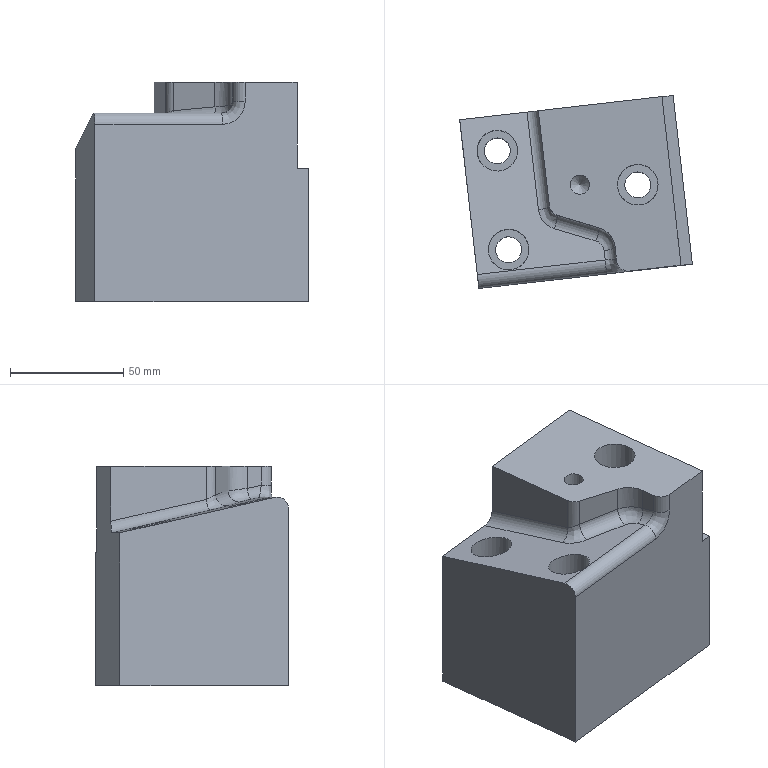Part | NX | features solid 2 | 1 solid | 37 faces | box 102.88 x 85.272 x 97 mm | volume 557494 mm3 | cylinder 16 | plane 15 | spline 3 | cone 3 | commonest cylinder face diameters 10 x6 8.5 x3 11.5 x3 18 x3 20 x1
STEP:
#1=CARTESIAN_POINT('',(2285.765,326.679,-55.281));
#2=VERTEX_POINT('',#1);
#3=CARTESIAN_POINT('',(2285.765,326.679,-31.));
#4=VERTEX_POINT('',#3);
#5=CARTESIAN_POINT('',(2285.765,326.679,-37.));
#6=DIRECTION('',(0.,0.,1.));
#7=VECTOR('',#6,1000.);
#8=LINE('',#5,#7);
#9=EDGE_CURVE('',#2,#4,#8,.T.);
#10=ORIENTED_EDGE('',*,*,#9,.T.);
#11=CARTESIAN_POINT('',(2340.433,332.908,-31.));
#12=VERTEX_POINT('',#11);
#13=CARTESIAN_POINT('',(2360.305,335.172,-31.));
#14=DIRECTION('',(0.9936,0.1132,0.));
#15=VECTOR('',#14,1000.);
#16=LINE('',#13,#15);
#17=EDGE_CURVE('',#4,#12,#16,.T.);
#18=ORIENTED_EDGE('',*,*,#17,.T.);
#19=CARTESIAN_POINT('',(2340.433,332.908,-69.));
#20=VERTEX_POINT('',#19);
#21=CARTESIAN_POINT('',(2340.433,332.908,-37.));
#22=DIRECTION('',(0.,0.,1.));
#23=VECTOR('',#22,1000.);
#24=LINE('',#21,#23);
#25=EDGE_CURVE('',#20,#12,#24,.T.);
#26=ORIENTED_EDGE('',*,*,#25,.F.);
#27=CARTESIAN_POINT('',(2345.401,333.474,-69.));
#28=VERTEX_POINT('',#27);
#29=CARTESIAN_POINT('',(2360.305,335.172,-69.));
#30=DIRECTION('',(0.9936,0.1132,0.));
#31=VECTOR('',#30,1000.);
#32=LINE('',#29,#31);
#33=EDGE_CURVE('',#20,#28,#32,.T.);
#34=ORIENTED_EDGE('',*,*,#33,.T.);
#35=CARTESIAN_POINT('',(2345.401,333.474,-128.));
#36=VERTEX_POINT('',#35);
#37=CARTESIAN_POINT('',(2345.401,333.474,-37.));
#38=DIRECTION('',(0.,0.,1.));
#39=VECTOR('',#38,1000.);
#40=LINE('',#37,#39);
#41=EDGE_CURVE('',#36,#28,#40,.T.);
#42=ORIENTED_EDGE('',*,*,#41,.F.);
#43=CARTESIAN_POINT('',(2251.012,322.719,-128.));
#44=VERTEX_POINT('',#43);
#45=CARTESIAN_POINT('',(2360.305,335.172,-128.));
#46=DIRECTION('',(0.9936,0.1132,0.));
#47=VECTOR('',#46,1000.);
#48=LINE('',#45,#47);
#49=EDGE_CURVE('',#44,#36,#48,.T.);
#50=ORIENTED_EDGE('',*,*,#49,.F.);
#51=CARTESIAN_POINT('',(2251.012,322.719,-60.413));
#52=VERTEX_POINT('',#51);
#53=CARTESIAN_POINT('',(2251.012,322.719,-45.));
#54=DIRECTION('',(0.,0.,-1.));
#55=VECTOR('',#54,1000.);
#56=LINE('',#53,#55);
#57=EDGE_CURVE('',#52,#44,#56,.T.);
#58=ORIENTED_EDGE('',*,*,#57,.F.);
#59=CARTESIAN_POINT('',(2280.794,326.113,-60.413));
#60=VERTEX_POINT('',#59);
#61=CARTESIAN_POINT('',(2360.305,335.172,-60.413));
#62=DIRECTION('',(0.9936,0.1132,-0.000000001));
#63=VECTOR('',#62,1000.);
#64=LINE('',#61,#63);
#65=EDGE_CURVE('',#52,#60,#64,.T.);
#66=ORIENTED_EDGE('',*,*,#65,.T.);
#67=CARTESIAN_POINT('',(2280.797,326.113,-55.285));
#68=DIRECTION('',(-0.1132,0.9936,0.));
#69=DIRECTION('',(-0.01222,-0.001392,-0.9999));
#70=AXIS2_PLACEMENT_3D('',#67,#68,#69);
#71=ELLIPSE('',#70,5.128,5.);
#72=EDGE_CURVE('',#2,#60,#71,.T.);
#73=ORIENTED_EDGE('',*,*,#72,.F.);
#74=EDGE_LOOP('',(#10,#18,#26,#34,#42,#50,#58,#66,#73));
#75=FACE_BOUND('',#74,.T.);
#76=CARTESIAN_POINT('',(2360.305,335.172,-37.));
#77=DIRECTION('',(-0.1132,0.9936,0.));
#78=DIRECTION('',(-0.9936,-0.1132,0.));
#79=AXIS2_PLACEMENT_3D('',#76,#77,#78);
#80=PLANE('',#79);
#81=ADVANCED_FACE('',(#75),#80,.T.);
#82=CARTESIAN_POINT('',(2316.03,254.642,-49.593));
#83=VERTEX_POINT('',#82);
#84=CARTESIAN_POINT('',(2325.966,255.774,-39.337));
#85=VERTEX_POINT('',#84);
#86=CARTESIAN_POINT('',(2316.03,254.642,-39.337));
#87=DIRECTION('',(0.1132,-0.9936,0.));
#88=DIRECTION('',(-0.0002839,-0.00003235,1.));
#89=AXIS2_PLACEMENT_3D('',#86,#87,#88);
#90=ELLIPSE('',#89,10.256,10.);
#91=EDGE_CURVE('',#83,#85,#90,.T.);
#92=ORIENTED_EDGE('',*,*,#91,.F.);
#93=CARTESIAN_POINT('',(2259.502,248.201,-49.593));
#94=VERTEX_POINT('',#93);
#95=CARTESIAN_POINT('',(2368.795,260.654,-49.593));
#96=DIRECTION('',(0.9936,0.1132,-0.000000001));
#97=VECTOR('',#96,1000.);
#98=LINE('',#95,#97);
#99=EDGE_CURVE('',#94,#83,#98,.T.);
#100=ORIENTED_EDGE('',*,*,#99,.F.);
#101=CARTESIAN_POINT('',(2259.502,248.201,-128.));
#102=VERTEX_POINT('',#101);
#103=CARTESIAN_POINT('',(2259.502,248.201,-45.));
#104=DIRECTION('',(0.,0.,1.));
#105=VECTOR('',#104,1000.);
#106=LINE('',#103,#105);
#107=EDGE_CURVE('',#102,#94,#106,.T.);
#108=ORIENTED_EDGE('',*,*,#107,.F.);
#109=CARTESIAN_POINT('',(2353.891,258.956,-128.));
#110=VERTEX_POINT('',#109);
#111=CARTESIAN_POINT('',(2329.052,256.126,-128.));
#112=DIRECTION('',(0.9936,0.1132,0.));
#113=VECTOR('',#112,1000.);
#114=LINE('',#111,#113);
#115=EDGE_CURVE('',#102,#110,#114,.T.);
#116=ORIENTED_EDGE('',*,*,#115,.T.);
#117=CARTESIAN_POINT('',(2353.891,258.956,-69.));
#118=VERTEX_POINT('',#117);
#119=CARTESIAN_POINT('',(2353.891,258.956,-74.));
#120=DIRECTION('',(0.,0.,1.));
#121=VECTOR('',#120,1000.);
#122=LINE('',#119,#121);
#123=EDGE_CURVE('',#110,#118,#122,.T.);
#124=ORIENTED_EDGE('',*,*,#123,.T.);
#125=CARTESIAN_POINT('',(2348.923,258.39,-69.));
#126=VERTEX_POINT('',#125);
#127=CARTESIAN_POINT('',(2353.891,258.956,-69.));
#128=DIRECTION('',(0.9936,0.1132,0.));
#129=VECTOR('',#128,1000.);
#130=LINE('',#127,#129);
#131=EDGE_CURVE('',#126,#118,#130,.T.);
#132=ORIENTED_EDGE('',*,*,#131,.F.);
#133=CARTESIAN_POINT('',(2348.923,258.39,-31.));
#134=VERTEX_POINT('',#133);
#135=CARTESIAN_POINT('',(2348.923,258.39,-37.));
#136=DIRECTION('',(0.,0.,-1.));
#137=VECTOR('',#136,1000.);
#138=LINE('',#135,#137);
#139=EDGE_CURVE('',#134,#126,#138,.T.);
#140=ORIENTED_EDGE('',*,*,#139,.F.);
#141=CARTESIAN_POINT('',(2325.966,255.774,-31.));
#142=VERTEX_POINT('',#141);
#143=CARTESIAN_POINT('',(2363.827,260.088,-31.));
#144=DIRECTION('',(0.9936,0.1132,0.));
#145=VECTOR('',#144,1000.);
#146=LINE('',#143,#145);
#147=EDGE_CURVE('',#142,#134,#146,.T.);
#148=ORIENTED_EDGE('',*,*,#147,.F.);
#149=CARTESIAN_POINT('',(2325.966,255.774,-256.));
#150=DIRECTION('',(0.,0.,1.));
#151=VECTOR('',#150,1000.);
#152=LINE('',#149,#151);
#153=EDGE_CURVE('',#85,#142,#152,.T.);
#154=ORIENTED_EDGE('',*,*,#153,.F.);
#155=EDGE_LOOP('',(#92,#100,#108,#116,#124,#132,#140,#148,#154));
#156=FACE_BOUND('',#155,.T.);
#157=CARTESIAN_POINT('',(2368.795,260.654,-37.));
#158=DIRECTION('',(0.1132,-0.9936,0.));
#159=DIRECTION('',(0.9936,0.1132,0.));
#160=AXIS2_PLACEMENT_3D('',#157,#158,#159);
#161=PLANE('',#160);
#162=ADVANCED_FACE('',(#156),#161,.T.);
#163=CARTESIAN_POINT('',(2308.389,293.991,-31.));
#164=VERTEX_POINT('',#163);
#165=CARTESIAN_POINT('',(2304.139,293.991,-31.));
#166=DIRECTION('',(0.,0.,1.));
#167=DIRECTION('',(1.,0.,0.));
#168=AXIS2_PLACEMENT_3D('',#165,#166,#167);
#169=CIRCLE('',#168,4.25);
#170=EDGE_CURVE('',#164,#164,#169,.T.);
#171=ORIENTED_EDGE('',*,*,#170,.F.);
#172=EDGE_LOOP('',(#171));
#173=FACE_BOUND('',#172,.T.);
#174=CARTESIAN_POINT('',(2338.775,293.951,-31.));
#175=VERTEX_POINT('',#174);
#176=CARTESIAN_POINT('',(2329.775,293.951,-31.));
#177=DIRECTION('',(0.,0.,1.));
#178=DIRECTION('',(1.,0.,0.));
#179=AXIS2_PLACEMENT_3D('',#176,#177,#178);
#180=CIRCLE('',#179,9.);
#181=EDGE_CURVE('',#175,#175,#180,.T.);
#182=ORIENTED_EDGE('',*,*,#181,.F.);
#183=EDGE_LOOP('',(#182));
#184=FACE_BOUND('',#183,.T.);
#185=CARTESIAN_POINT('',(2312.617,274.947,-31.));
#186=VERTEX_POINT('',#185);
#187=CARTESIAN_POINT('',(2294.224,280.394,-31.));
#188=VERTEX_POINT('',#187);
#189=CARTESIAN_POINT('',(2363.743,259.806,-31.));
#190=DIRECTION('',(-0.9588,0.284,0.));
#191=VECTOR('',#190,1000.);
#192=LINE('',#189,#191);
#193=EDGE_CURVE('',#186,#188,#192,.T.);
#194=ORIENTED_EDGE('',*,*,#193,.F.);
#195=CARTESIAN_POINT('',(2319.713,266.49,-31.));
#196=VERTEX_POINT('',#195);
#197=CARTESIAN_POINT('',(2309.777,265.358,-31.));
#198=DIRECTION('',(0.,0.,-1.));
#199=DIRECTION('',(1.,0.,0.));
#200=AXIS2_PLACEMENT_3D('',#197,#198,#199);
#201=CIRCLE('',#200,10.);
#202=EDGE_CURVE('',#186,#196,#201,.T.);
#203=ORIENTED_EDGE('',*,*,#202,.T.);
#204=CARTESIAN_POINT('',(2320.432,260.176,-31.));
#205=VERTEX_POINT('',#204);
#206=CARTESIAN_POINT('',(2320.997,255.211,-31.));
#207=DIRECTION('',(-0.1131,0.9936,0.));
#208=VECTOR('',#207,1000.);
#209=LINE('',#206,#208);
#210=EDGE_CURVE('',#205,#196,#209,.T.);
#211=ORIENTED_EDGE('',*,*,#210,.F.);
#212=CARTESIAN_POINT('',(2325.4,260.742,-31.));
#213=DIRECTION('',(0.,0.,-1.));
#214=DIRECTION('',(1.,0.,0.));
#215=AXIS2_PLACEMENT_3D('',#212,#213,#214);
#216=CIRCLE('',#215,5.);
#217=EDGE_CURVE('',#142,#205,#216,.T.);
#218=ORIENTED_EDGE('',*,*,#217,.F.);
#219=ORIENTED_EDGE('',*,*,#147,.T.);
#220=CARTESIAN_POINT('',(2348.923,258.39,-31.));
#221=DIRECTION('',(-0.1132,0.9936,0.));
#222=VECTOR('',#221,1000.);
#223=LINE('',#220,#222);
#224=EDGE_CURVE('',#134,#12,#223,.T.);
#225=ORIENTED_EDGE('',*,*,#224,.T.);
#226=ORIENTED_EDGE('',*,*,#17,.F.);
#227=CARTESIAN_POINT('',(2290.677,284.608,-31.));
#228=VERTEX_POINT('',#227);
#229=CARTESIAN_POINT('',(2291.366,278.709,-31.));
#230=DIRECTION('',(0.116,-0.9933,0.));
#231=VECTOR('',#230,1000.);
#232=LINE('',#229,#231);
#233=EDGE_CURVE('',#4,#228,#232,.T.);
#234=ORIENTED_EDGE('',*,*,#233,.T.);
#235=CARTESIAN_POINT('',(2295.644,285.188,-31.));
#236=DIRECTION('',(0.,0.,-1.));
#237=DIRECTION('',(1.,0.,0.));
#238=AXIS2_PLACEMENT_3D('',#235,#236,#237);
#239=CIRCLE('',#238,5.);
#240=EDGE_CURVE('',#188,#228,#239,.T.);
#241=ORIENTED_EDGE('',*,*,#240,.F.);
#242=EDGE_LOOP('',(#194,#203,#211,#218,#219,#225,#226,#234,#241));
#243=FACE_BOUND('',#242,.T.);
#244=CARTESIAN_POINT('',(2363.827,260.088,-31.));
#245=DIRECTION('',(0.,0.,1.));
#246=DIRECTION('',(-0.1132,0.9936,0.));
#247=AXIS2_PLACEMENT_3D('',#244,#245,#246);
#248=PLANE('',#247);
#249=ADVANCED_FACE('',(#173,#184,#243),#248,.T.);
#250=CARTESIAN_POINT('',(2259.502,248.201,-128.));
#251=DIRECTION('',(-0.1132,0.9936,0.));
#252=VECTOR('',#251,1000.);
#253=LINE('',#250,#252);
#254=EDGE_CURVE('',#102,#44,#253,.T.);
#255=ORIENTED_EDGE('',*,*,#254,.T.);
#256=ORIENTED_EDGE('',*,*,#49,.T.);
#257=CARTESIAN_POINT('',(2353.891,258.956,-128.));
#258=DIRECTION('',(-0.1132,0.9936,0.));
#259=VECTOR('',#258,1000.);
#260=LINE('',#257,#259);
#261=EDGE_CURVE('',#110,#36,#260,.T.);
#262=ORIENTED_EDGE('',*,*,#261,.F.);
#263=ORIENTED_EDGE('',*,*,#115,.F.);
#264=EDGE_LOOP('',(#255,#256,#262,#263));
#265=FACE_BOUND('',#264,.T.);
#266=CARTESIAN_POINT('',(2335.488,294.602,-128.));
#267=VERTEX_POINT('',#266);
#268=CARTESIAN_POINT('',(2329.775,293.951,-128.));
#269=DIRECTION('',(0.,0.,-1.));
#270=DIRECTION('',(0.9936,0.1132,0.));
#271=AXIS2_PLACEMENT_3D('',#268,#269,#270);
#272=CIRCLE('',#271,5.75);
#273=EDGE_CURVE('',#267,#267,#272,.T.);
#274=ORIENTED_EDGE('',*,*,#273,.F.);
#275=EDGE_LOOP('',(#274));
#276=FACE_BOUND('',#275,.T.);
#277=CARTESIAN_POINT('',(2273.42,309.017,-128.));
#278=VERTEX_POINT('',#277);
#279=CARTESIAN_POINT('',(2267.67,309.017,-128.));
#280=DIRECTION('',(0.,0.,-1.));
#281=DIRECTION('',(1.,0.,0.));
#282=AXIS2_PLACEMENT_3D('',#279,#280,#281);
#283=CIRCLE('',#282,5.75);
#284=EDGE_CURVE('',#278,#278,#283,.T.);
#285=ORIENTED_EDGE('',*,*,#284,.F.);
#286=EDGE_LOOP('',(#285));
#287=FACE_BOUND('',#286,.T.);
#288=CARTESIAN_POINT('',(2278.364,265.951,-128.));
#289=VERTEX_POINT('',#288);
#290=CARTESIAN_POINT('',(2272.651,265.3,-128.));
#291=DIRECTION('',(0.,0.,1.));
#292=DIRECTION('',(0.9936,0.1132,0.));
#293=AXIS2_PLACEMENT_3D('',#290,#291,#292);
#294=CIRCLE('',#293,5.75);
#295=EDGE_CURVE('',#289,#289,#294,.T.);
#296=ORIENTED_EDGE('',*,*,#295,.T.);
#297=EDGE_LOOP('',(#296));
#298=FACE_BOUND('',#297,.T.);
#299=CARTESIAN_POINT('',(2329.052,256.126,-128.));
#300=DIRECTION('',(0.,0.,1.));
#301=DIRECTION('',(-0.9936,-0.1132,0.));
#302=AXIS2_PLACEMENT_3D('',#299,#300,#301);
#303=PLANE('',#302);
#304=ADVANCED_FACE('',(#265,#276,#287,#298),#303,.F.);
#305=CARTESIAN_POINT('',(2324.062,293.3,-98.));
#306=VERTEX_POINT('',#305);
#307=CARTESIAN_POINT('',(2329.775,293.951,-98.));
#308=DIRECTION('',(0.,0.,1.));
#309=DIRECTION('',(-0.9936,-0.1132,0.));
#310=AXIS2_PLACEMENT_3D('',#307,#308,#309);
#311=CIRCLE('',#310,5.75);
#312=EDGE_CURVE('',#306,#306,#311,.T.);
#313=ORIENTED_EDGE('',*,*,#312,.F.);
#314=EDGE_LOOP('',(#313));
#315=FACE_BOUND('',#314,.T.);
#316=CARTESIAN_POINT('',(2338.717,294.969,-98.));
#317=VERTEX_POINT('',#316);
#318=CARTESIAN_POINT('',(2329.775,293.951,-98.));
#319=DIRECTION('',(0.,0.,1.));
#320=DIRECTION('',(0.9936,0.1132,0.));
#321=AXIS2_PLACEMENT_3D('',#318,#319,#320);
#322=CIRCLE('',#321,9.);
#323=EDGE_CURVE('',#317,#317,#322,.T.);
#324=ORIENTED_EDGE('',*,*,#323,.T.);
#325=EDGE_LOOP('',(#324));
#326=FACE_BOUND('',#325,.T.);
#327=CARTESIAN_POINT('',(2329.775,293.951,-98.));
#328=DIRECTION('',(0.,0.,-1.));
#329=DIRECTION('',(0.9936,0.1132,0.));
#330=AXIS2_PLACEMENT_3D('',#327,#328,#329);
#331=PLANE('',#330);
#332=ADVANCED_FACE('',(#315,#326),#331,.F.);
#333=ORIENTED_EDGE('',*,*,#131,.T.);
#334=CARTESIAN_POINT('',(2353.891,258.956,-69.));
#335=DIRECTION('',(-0.1132,0.9936,0.));
#336=VECTOR('',#335,1000.);
#337=LINE('',#334,#336);
#338=EDGE_CURVE('',#118,#28,#337,.T.);
#339=ORIENTED_EDGE('',*,*,#338,.T.);
#340=ORIENTED_EDGE('',*,*,#33,.F.);
#341=CARTESIAN_POINT('',(2348.923,258.39,-69.));
#342=DIRECTION('',(-0.1132,0.9936,0.));
#343=VECTOR('',#342,1000.);
#344=LINE('',#341,#343);
#345=EDGE_CURVE('',#126,#20,#344,.T.);
#346=ORIENTED_EDGE('',*,*,#345,.F.);
#347=EDGE_LOOP('',(#333,#339,#340,#346));
#348=FACE_BOUND('',#347,.T.);
#349=CARTESIAN_POINT('',(2353.891,258.956,-69.));
#350=DIRECTION('',(0.,0.,-1.));
#351=DIRECTION('',(0.1132,-0.9936,0.));
#352=AXIS2_PLACEMENT_3D('',#349,#350,#351);
#353=PLANE('',#352);
#354=ADVANCED_FACE('',(#348),#353,.F.);
#355=ORIENTED_EDGE('',*,*,#312,.T.);
#356=EDGE_LOOP('',(#355));
#357=FACE_BOUND('',#356,.T.);
#358=ORIENTED_EDGE('',*,*,#273,.T.);
#359=EDGE_LOOP('',(#358));
#360=FACE_BOUND('',#359,.T.);
#361=CARTESIAN_POINT('',(2329.775,293.951,-5.));
#362=DIRECTION('',(0.,0.,-1.));
#363=DIRECTION('',(-0.9936,-0.1132,0.));
#364=AXIS2_PLACEMENT_3D('',#361,#362,#363);
#365=CYLINDRICAL_SURFACE('',#364,5.75);
#366=ADVANCED_FACE('',(#357,#360),#365,.F.);
#367=ORIENTED_EDGE('',*,*,#338,.F.);
#368=ORIENTED_EDGE('',*,*,#123,.F.);
#369=ORIENTED_EDGE('',*,*,#261,.T.);
#370=ORIENTED_EDGE('',*,*,#41,.T.);
#371=EDGE_LOOP('',(#367,#368,#369,#370));
#372=FACE_BOUND('',#371,.T.);
#373=CARTESIAN_POINT('',(2353.891,258.956,-74.));
#374=DIRECTION('',(-0.9936,-0.1132,0.));
#375=DIRECTION('',(0.,0.,-1.));
#376=AXIS2_PLACEMENT_3D('',#373,#374,#375);
#377=PLANE('',#376);
#378=ADVANCED_FACE('',(#372),#377,.F.);
#379=ORIENTED_EDGE('',*,*,#323,.F.);
#380=EDGE_LOOP('',(#379));
#381=FACE_BOUND('',#380,.T.);
#382=ORIENTED_EDGE('',*,*,#181,.T.);
#383=EDGE_LOOP('',(#382));
#384=FACE_BOUND('',#383,.T.);
#385=CARTESIAN_POINT('',(2329.775,293.951,-26.));
#386=DIRECTION('',(0.,0.,-1.));
#387=DIRECTION('',(-0.9936,-0.1132,0.));
#388=AXIS2_PLACEMENT_3D('',#385,#386,#387);
#389=CYLINDRICAL_SURFACE('',#388,9.);
#390=ADVANCED_FACE('',(#381,#384),#389,.F.);
#391=CARTESIAN_POINT('',(2347.28,272.815,-45.777));
#392=VERTEX_POINT('',#391);
#393=CARTESIAN_POINT('',(2347.225,273.293,-50.));
#394=DIRECTION('',(-0.9936,-0.1132,0.));
#395=DIRECTION('',(0.01281,-0.1125,0.9936));
#396=AXIS2_PLACEMENT_3D('',#393,#394,#395);
#397=CIRCLE('',#396,4.25);
#398=EDGE_CURVE('',#392,#392,#397,.T.);
#399=ORIENTED_EDGE('',*,*,#398,.T.);
#400=EDGE_LOOP('',(#399));
#401=FACE_BOUND('',#400,.T.);
#402=CARTESIAN_POINT('',(2342.186,317.526,-45.777));
#403=VERTEX_POINT('',#402);
#404=CARTESIAN_POINT('',(2342.131,318.004,-50.));
#405=DIRECTION('',(-0.9936,-0.1132,0.));
#406=DIRECTION('',(0.01281,-0.1125,0.9936));
#407=AXIS2_PLACEMENT_3D('',#404,#405,#406);
#408=CIRCLE('',#407,4.25);
#409=EDGE_CURVE('',#403,#403,#408,.T.);
#410=ORIENTED_EDGE('',*,*,#409,.T.);
#411=EDGE_LOOP('',(#410));
#412=FACE_BOUND('',#411,.T.);
#413=ORIENTED_EDGE('',*,*,#25,.T.);
#414=ORIENTED_EDGE('',*,*,#224,.F.);
#415=ORIENTED_EDGE('',*,*,#139,.T.);
#416=ORIENTED_EDGE('',*,*,#345,.T.);
#417=EDGE_LOOP('',(#413,#414,#415,#416));
#418=FACE_BOUND('',#417,.T.);
#419=CARTESIAN_POINT('',(2348.923,258.39,-45.));
#420=DIRECTION('',(-0.9936,-0.1132,0.));
#421=DIRECTION('',(0.1132,-0.9936,0.));
#422=AXIS2_PLACEMENT_3D('',#419,#420,#421);
#423=PLANE('',#422);
#424=ADVANCED_FACE('',(#401,#412,#418),#423,.F.);
#425=CARTESIAN_POINT('',(2319.713,266.49,-40.785));
#426=VERTEX_POINT('',#425);
#427=CARTESIAN_POINT('',(2319.713,266.49,-256.));
#428=DIRECTION('',(0.,0.,1.));
#429=VECTOR('',#428,1000.);
#430=LINE('',#427,#429);
#431=EDGE_CURVE('',#426,#196,#430,.T.);
#432=ORIENTED_EDGE('',*,*,#431,.T.);
#433=ORIENTED_EDGE('',*,*,#202,.F.);
#434=CARTESIAN_POINT('',(2312.617,274.947,-41.833));
#435=VERTEX_POINT('',#434);
#436=CARTESIAN_POINT('',(2312.617,274.947,-256.));
#437=DIRECTION('',(0.,0.,1.));
#438=VECTOR('',#437,1000.);
#439=LINE('',#436,#438);
#440=EDGE_CURVE('',#435,#186,#439,.T.);
#441=ORIENTED_EDGE('',*,*,#440,.F.);
#442=CARTESIAN_POINT('',(2312.617,274.947,-41.833));
#443=CARTESIAN_POINT('',(2313.475,274.692,-41.794));
#444=CARTESIAN_POINT('',(2314.773,274.117,-41.711));
#445=CARTESIAN_POINT('',(2316.168,273.08,-41.576));
#446=CARTESIAN_POINT('',(2316.827,272.457,-41.497));
#447=CARTESIAN_POINT('',(2317.174,272.093,-41.452));
#448=CARTESIAN_POINT('',(2317.466,271.756,-41.41));
#449=CARTESIAN_POINT('',(2317.59,271.601,-41.391));
#450=CARTESIAN_POINT('',(2317.822,271.304,-41.354));
#451=CARTESIAN_POINT('',(2318.209,270.759,-41.286));
#452=CARTESIAN_POINT('',(2319.01,269.402,-41.121));
#453=CARTESIAN_POINT('',(2319.567,267.773,-40.932));
#454=CARTESIAN_POINT('',(2319.713,266.49,-40.785));
#455=B_SPLINE_CURVE_WITH_KNOTS('',3,(#442,#443,#444,#445,#446,#447,#448,#449,#450,#451,#452,#453,#454),.UNSPECIFIED.,.F.,.F.,(4,1,1,1,1,1,1,1,1,1,4),(0.,0.25,0.375,0.4375,0.4688,0.5,0.5312,0.5625,0.625,0.75,1.),.UNSPECIFIED.);
#456=EDGE_CURVE('',#426,#435,#455,.F.);
#457=ORIENTED_EDGE('',*,*,#456,.F.);
#458=EDGE_LOOP('',(#432,#433,#441,#457));
#459=FACE_BOUND('',#458,.T.);
#460=CARTESIAN_POINT('',(2309.777,265.358,-256.));
#461=DIRECTION('',(0.,0.,1.));
#462=DIRECTION('',(-1.,0.,0.));
#463=AXIS2_PLACEMENT_3D('',#460,#461,#462);
#464=CYLINDRICAL_SURFACE('',#463,10.);
#465=ADVANCED_FACE('',(#459),#464,.F.);
#466=CARTESIAN_POINT('',(2294.224,280.394,-43.541));
#467=VERTEX_POINT('',#466);
#468=CARTESIAN_POINT('',(2290.537,281.485,-43.883));
#469=DIRECTION('',(-0.9551,0.2828,-0.08865));
#470=VECTOR('',#469,1000.);
#471=LINE('',#468,#470);
#472=EDGE_CURVE('',#435,#467,#471,.T.);
#473=ORIENTED_EDGE('',*,*,#472,.F.);
#474=ORIENTED_EDGE('',*,*,#440,.T.);
#475=ORIENTED_EDGE('',*,*,#193,.T.);
#476=CARTESIAN_POINT('',(2294.224,280.394,-256.));
#477=DIRECTION('',(0.,0.,1.));
#478=VECTOR('',#477,1000.);
#479=LINE('',#476,#478);
#480=EDGE_CURVE('',#467,#188,#479,.T.);
#481=ORIENTED_EDGE('',*,*,#480,.F.);
#482=EDGE_LOOP('',(#473,#474,#475,#481));
#483=FACE_BOUND('',#482,.T.);
#484=CARTESIAN_POINT('',(2312.617,274.947,-256.));
#485=DIRECTION('',(-0.284,-0.9588,0.));
#486=DIRECTION('',(0.9588,-0.284,0.));
#487=AXIS2_PLACEMENT_3D('',#484,#485,#486);
#488=PLANE('',#487);
#489=ADVANCED_FACE('',(#483),#488,.T.);
#490=ORIENTED_EDGE('',*,*,#210,.T.);
#491=ORIENTED_EDGE('',*,*,#431,.F.);
#492=CARTESIAN_POINT('',(2320.432,260.176,-39.337));
#493=VERTEX_POINT('',#492);
#494=CARTESIAN_POINT('',(2319.587,267.593,-41.038));
#495=DIRECTION('',(-0.1103,0.9688,-0.2221));
#496=VECTOR('',#495,1000.);
#497=LINE('',#494,#496);
#498=EDGE_CURVE('',#493,#426,#497,.T.);
#499=ORIENTED_EDGE('',*,*,#498,.F.);
#500=CARTESIAN_POINT('',(2320.432,260.176,-43.326));
#501=DIRECTION('',(0.,0.,-1.));
#502=VECTOR('',#501,1000.);
#503=LINE('',#500,#502);
#504=EDGE_CURVE('',#205,#493,#503,.T.);
#505=ORIENTED_EDGE('',*,*,#504,.F.);
#506=EDGE_LOOP('',(#490,#491,#499,#505));
#507=FACE_BOUND('',#506,.T.);
#508=CARTESIAN_POINT('',(2321.836,247.849,-256.));
#509=DIRECTION('',(-0.9936,-0.1131,0.));
#510=DIRECTION('',(0.1131,-0.9936,0.));
#511=AXIS2_PLACEMENT_3D('',#508,#509,#510);
#512=PLANE('',#511);
#513=ADVANCED_FACE('',(#507),#512,.T.);
#514=ORIENTED_EDGE('',*,*,#233,.F.);
#515=ORIENTED_EDGE('',*,*,#9,.F.);
#516=CARTESIAN_POINT('',(2290.677,284.608,-45.632));
#517=VERTEX_POINT('',#516);
#518=CARTESIAN_POINT('',(2287.781,309.407,-51.32));
#519=DIRECTION('',(-0.1131,0.9684,-0.2221));
#520=VECTOR('',#519,1000.);
#521=LINE('',#518,#520);
#522=EDGE_CURVE('',#517,#2,#521,.T.);
#523=ORIENTED_EDGE('',*,*,#522,.F.);
#524=CARTESIAN_POINT('',(2290.677,284.608,-256.));
#525=DIRECTION('',(0.,0.,-1.));
#526=VECTOR('',#525,1000.);
#527=LINE('',#524,#526);
#528=EDGE_CURVE('',#228,#517,#527,.T.);
#529=ORIENTED_EDGE('',*,*,#528,.F.);
#530=EDGE_LOOP('',(#514,#515,#523,#529));
#531=FACE_BOUND('',#530,.T.);
#532=CARTESIAN_POINT('',(2291.366,278.709,-256.));
#533=DIRECTION('',(-0.9933,-0.116,0.));
#534=DIRECTION('',(0.116,-0.9933,0.));
#535=AXIS2_PLACEMENT_3D('',#532,#533,#534);
#536=PLANE('',#535);
#537=ADVANCED_FACE('',(#531),#536,.T.);
#538=CARTESIAN_POINT('',(2278.364,265.951,-98.));
#539=VERTEX_POINT('',#538);
#540=CARTESIAN_POINT('',(2272.651,265.3,-98.));
#541=DIRECTION('',(0.,0.,-1.));
#542=DIRECTION('',(0.9936,0.1132,0.));
#543=AXIS2_PLACEMENT_3D('',#540,#541,#542);
#544=CIRCLE('',#543,5.75);
#545=EDGE_CURVE('',#539,#539,#544,.T.);
#546=ORIENTED_EDGE('',*,*,#545,.T.);
#547=EDGE_LOOP('',(#546));
#548=FACE_BOUND('',#547,.T.);
#549=CARTESIAN_POINT('',(2263.709,264.281,-98.));
#550=VERTEX_POINT('',#549);
#551=CARTESIAN_POINT('',(2272.651,265.3,-98.));
#552=DIRECTION('',(0.,0.,-1.));
#553=DIRECTION('',(-0.9936,-0.1132,0.));
#554=AXIS2_PLACEMENT_3D('',#551,#552,#553);
#555=CIRCLE('',#554,9.);
#556=EDGE_CURVE('',#550,#550,#555,.T.);
#557=ORIENTED_EDGE('',*,*,#556,.F.);
#558=EDGE_LOOP('',(#557));
#559=FACE_BOUND('',#558,.T.);
#560=CARTESIAN_POINT('',(2272.651,265.3,-98.));
#561=DIRECTION('',(0.,0.,-1.));
#562=DIRECTION('',(-0.9936,-0.1132,0.));
#563=AXIS2_PLACEMENT_3D('',#560,#561,#562);
#564=PLANE('',#563);
#565=ADVANCED_FACE('',(#548,#559),#564,.F.);
#566=CARTESIAN_POINT('',(2273.383,309.668,-98.));
#567=VERTEX_POINT('',#566);
#568=CARTESIAN_POINT('',(2267.67,309.017,-98.));
#569=DIRECTION('',(0.,0.,-1.));
#570=DIRECTION('',(0.9936,0.1132,0.));
#571=AXIS2_PLACEMENT_3D('',#568,#569,#570);
#572=CIRCLE('',#571,5.75);
#573=EDGE_CURVE('',#567,#567,#572,.T.);
#574=ORIENTED_EDGE('',*,*,#573,.T.);
#575=EDGE_LOOP('',(#574));
#576=FACE_BOUND('',#575,.T.);
#577=CARTESIAN_POINT('',(2258.728,307.998,-98.));
#578=VERTEX_POINT('',#577);
#579=CARTESIAN_POINT('',(2267.67,309.017,-98.));
#580=DIRECTION('',(0.,0.,-1.));
#581=DIRECTION('',(-0.9936,-0.1132,0.));
#582=AXIS2_PLACEMENT_3D('',#579,#580,#581);
#583=CIRCLE('',#582,9.);
#584=EDGE_CURVE('',#578,#578,#583,.T.);
#585=ORIENTED_EDGE('',*,*,#584,.F.);
#586=EDGE_LOOP('',(#585));
#587=FACE_BOUND('',#586,.T.);
#588=CARTESIAN_POINT('',(2267.67,309.017,-98.));
#589=DIRECTION('',(0.,0.,-1.));
#590=DIRECTION('',(-0.9936,-0.1132,0.));
#591=AXIS2_PLACEMENT_3D('',#588,#589,#590);
#592=PLANE('',#591);
#593=ADVANCED_FACE('',(#576,#587),#592,.F.);
#594=ORIENTED_EDGE('',*,*,#584,.T.);
#595=EDGE_LOOP('',(#594));
#596=FACE_BOUND('',#595,.T.);
#597=CARTESIAN_POINT('',(2266.651,317.959,-58.932));
#598=VERTEX_POINT('',#597);
#599=CARTESIAN_POINT('',(2267.67,309.017,-56.881));
#600=DIRECTION('',(0.02515,-0.2207,-0.975));
#601=DIRECTION('',(-0.1104,0.9687,-0.2221));
#602=AXIS2_PLACEMENT_3D('',#599,#600,#601);
#603=ELLIPSE('',#602,9.231,9.);
#604=EDGE_CURVE('',#598,#598,#603,.T.);
#605=ORIENTED_EDGE('',*,*,#604,.F.);
#606=EDGE_LOOP('',(#605));
#607=FACE_BOUND('',#606,.T.);
#608=CARTESIAN_POINT('',(2267.67,309.017,-26.));
#609=DIRECTION('',(0.,0.,-1.));
#610=DIRECTION('',(0.9936,0.1132,0.));
#611=AXIS2_PLACEMENT_3D('',#608,#609,#610);
#612=CYLINDRICAL_SURFACE('',#611,9.);
#613=ADVANCED_FACE('',(#596,#607),#612,.F.);
#614=ORIENTED_EDGE('',*,*,#556,.T.);
#615=EDGE_LOOP('',(#614));
#616=FACE_BOUND('',#615,.T.);
#617=CARTESIAN_POINT('',(2271.632,274.242,-48.908));
#618=VERTEX_POINT('',#617);
#619=CARTESIAN_POINT('',(2272.651,265.3,-46.857));
#620=DIRECTION('',(0.02515,-0.2207,-0.975));
#621=DIRECTION('',(-0.1104,0.9687,-0.2221));
#622=AXIS2_PLACEMENT_3D('',#619,#620,#621);
#623=ELLIPSE('',#622,9.231,9.);
#624=EDGE_CURVE('',#618,#618,#623,.T.);
#625=ORIENTED_EDGE('',*,*,#624,.F.);
#626=EDGE_LOOP('',(#625));
#627=FACE_BOUND('',#626,.T.);
#628=CARTESIAN_POINT('',(2272.651,265.3,-26.));
#629=DIRECTION('',(0.,0.,-1.));
#630=DIRECTION('',(0.9936,0.1132,0.));
#631=AXIS2_PLACEMENT_3D('',#628,#629,#630);
#632=CYLINDRICAL_SURFACE('',#631,9.);
#633=ADVANCED_FACE('',(#616,#627),#632,.F.);
#634=ORIENTED_EDGE('',*,*,#545,.F.);
#635=EDGE_LOOP('',(#634));
#636=FACE_BOUND('',#635,.T.);
#637=ORIENTED_EDGE('',*,*,#295,.F.);
#638=EDGE_LOOP('',(#637));
#639=FACE_BOUND('',#638,.T.);
#640=CARTESIAN_POINT('',(2272.651,265.3,-5.));
#641=DIRECTION('',(0.,0.,-1.));
#642=DIRECTION('',(0.9936,0.1132,0.));
#643=AXIS2_PLACEMENT_3D('',#640,#641,#642);
#644=CYLINDRICAL_SURFACE('',#643,5.75);
#645=ADVANCED_FACE('',(#636,#639),#644,.F.);
#646=CARTESIAN_POINT('',(2258.81,254.273,-44.718));
#647=VERTEX_POINT('',#646);
#648=CARTESIAN_POINT('',(2244.589,379.096,-73.339));
#649=DIRECTION('',(-0.1104,0.9687,-0.2221));
#650=VECTOR('',#649,1000.);
#651=LINE('',#648,#650);
#652=EDGE_CURVE('',#647,#52,#651,.T.);
#653=ORIENTED_EDGE('',*,*,#652,.T.);
#654=ORIENTED_EDGE('',*,*,#57,.T.);
#655=ORIENTED_EDGE('',*,*,#254,.F.);
#656=ORIENTED_EDGE('',*,*,#107,.T.);
#657=CARTESIAN_POINT('',(2258.936,253.169,-49.593));
#658=DIRECTION('',(0.9936,0.1132,0.));
#659=DIRECTION('',(-0.1132,0.9936,0.));
#660=AXIS2_PLACEMENT_3D('',#657,#658,#659);
#661=CIRCLE('',#660,5.);
#662=EDGE_CURVE('',#647,#94,#661,.T.);
#663=ORIENTED_EDGE('',*,*,#662,.F.);
#664=EDGE_LOOP('',(#653,#654,#655,#656,#663));
#665=FACE_BOUND('',#664,.T.);
#666=CARTESIAN_POINT('',(2259.502,248.201,-45.));
#667=DIRECTION('',(-0.9936,-0.1132,0.));
#668=DIRECTION('',(0.1132,-0.9936,0.));
#669=AXIS2_PLACEMENT_3D('',#666,#667,#668);
#670=PLANE('',#669);
#671=ADVANCED_FACE('',(#665),#670,.T.);
#672=ORIENTED_EDGE('',*,*,#573,.F.);
#673=EDGE_LOOP('',(#672));
#674=FACE_BOUND('',#673,.T.);
#675=ORIENTED_EDGE('',*,*,#284,.T.);
#676=EDGE_LOOP('',(#675));
#677=FACE_BOUND('',#676,.T.);
#678=CARTESIAN_POINT('',(2267.67,309.017,-5.));
#679=DIRECTION('',(0.,0.,-1.));
#680=DIRECTION('',(0.9936,0.1132,0.));
#681=AXIS2_PLACEMENT_3D('',#678,#679,#680);
#682=CYLINDRICAL_SURFACE('',#681,5.75);
#683=ADVANCED_FACE('',(#674,#677),#682,.F.);
#684=ORIENTED_EDGE('',*,*,#65,.F.);
#685=ORIENTED_EDGE('',*,*,#652,.F.);
#686=CARTESIAN_POINT('',(2315.339,260.713,-44.718));
#687=VERTEX_POINT('',#686);
#688=CARTESIAN_POINT('',(2258.81,254.273,-44.718));
#689=DIRECTION('',(-0.9936,-0.1132,0.000000001));
#690=VECTOR('',#689,1000.);
#691=LINE('',#688,#690);
#692=EDGE_CURVE('',#687,#647,#691,.T.);
#693=ORIENTED_EDGE('',*,*,#692,.F.);
#694=CARTESIAN_POINT('',(2314.871,264.82,-45.66));
#695=VERTEX_POINT('',#694);
#696=CARTESIAN_POINT('',(2316.03,254.642,-43.326));
#697=DIRECTION('',(0.1103,-0.9688,0.2221));
#698=VECTOR('',#697,1000.);
#699=LINE('',#696,#698);
#700=EDGE_CURVE('',#695,#687,#699,.T.);
#701=ORIENTED_EDGE('',*,*,#700,.F.);
#702=CARTESIAN_POINT('',(2311.323,269.049,-46.709));
#703=VERTEX_POINT('',#702);
#704=CARTESIAN_POINT('',(2309.903,264.255,-45.66));
#705=DIRECTION('',(0.02515,-0.2207,-0.975));
#706=DIRECTION('',(0.1104,-0.9687,0.2221));
#707=AXIS2_PLACEMENT_3D('',#704,#705,#706);
#708=ELLIPSE('',#707,5.128,5.);
#709=EDGE_CURVE('',#703,#695,#708,.T.);
#710=ORIENTED_EDGE('',*,*,#709,.F.);
#711=CARTESIAN_POINT('',(2292.93,274.496,-48.416));
#712=VERTEX_POINT('',#711);
#713=CARTESIAN_POINT('',(2310.8,269.204,-46.757));
#714=DIRECTION('',(0.9551,-0.2828,0.08865));
#715=VECTOR('',#714,1000.);
#716=LINE('',#713,#715);
#717=EDGE_CURVE('',#712,#703,#716,.T.);
#718=ORIENTED_EDGE('',*,*,#717,.F.);
#719=CARTESIAN_POINT('',(2285.837,282.924,-50.507));
#720=VERTEX_POINT('',#719);
#721=CARTESIAN_POINT('',(2295.769,284.084,-50.513));
#722=DIRECTION('',(0.02515,-0.2207,-0.975));
#723=DIRECTION('',(0.1104,-0.9687,0.2221));
#724=AXIS2_PLACEMENT_3D('',#721,#722,#723);
#725=ELLIPSE('',#724,10.256,10.);
#726=EDGE_CURVE('',#712,#720,#725,.T.);
#727=ORIENTED_EDGE('',*,*,#726,.T.);
#728=CARTESIAN_POINT('',(2286.091,280.751,-50.008));
#729=DIRECTION('',(0.1131,-0.9684,0.2221));
#730=VECTOR('',#729,1000.);
#731=LINE('',#728,#730);
#732=EDGE_CURVE('',#60,#720,#731,.T.);
#733=ORIENTED_EDGE('',*,*,#732,.F.);
#734=EDGE_LOOP('',(#684,#685,#693,#701,#710,#718,#727,#733));
#735=FACE_BOUND('',#734,.T.);
#736=ORIENTED_EDGE('',*,*,#624,.T.);
#737=EDGE_LOOP('',(#736));
#738=FACE_BOUND('',#737,.T.);
#739=ORIENTED_EDGE('',*,*,#604,.T.);
#740=EDGE_LOOP('',(#739));
#741=FACE_BOUND('',#740,.T.);
#742=CARTESIAN_POINT('',(2253.256,380.083,-73.339));
#743=DIRECTION('',(0.02515,-0.2207,-0.975));
#744=DIRECTION('',(-0.1104,0.9687,-0.2221));
#745=AXIS2_PLACEMENT_3D('',#742,#743,#744);
#746=PLANE('',#745);
#747=ADVANCED_FACE('',(#735,#738,#741),#746,.F.);
#748=ORIENTED_EDGE('',*,*,#662,.T.);
#749=ORIENTED_EDGE('',*,*,#99,.T.);
#750=CARTESIAN_POINT('',(2315.464,259.61,-49.593));
#751=DIRECTION('',(-0.9936,-0.1132,0.000000001));
#752=DIRECTION('',(-0.1132,0.9936,0.));
#753=AXIS2_PLACEMENT_3D('',#750,#751,#752);
#754=CIRCLE('',#753,5.);
#755=EDGE_CURVE('',#83,#687,#754,.T.);
#756=ORIENTED_EDGE('',*,*,#755,.T.);
#757=ORIENTED_EDGE('',*,*,#692,.T.);
#758=EDGE_LOOP('',(#748,#749,#756,#757));
#759=FACE_BOUND('',#758,.T.);
#760=CARTESIAN_POINT('',(2368.229,265.622,-49.593));
#761=DIRECTION('',(-0.9936,-0.1132,0.000000001));
#762=DIRECTION('',(0.1132,-0.9936,0.));
#763=AXIS2_PLACEMENT_3D('',#760,#761,#762);
#764=CYLINDRICAL_SURFACE('',#763,5.);
#765=ADVANCED_FACE('',(#759),#764,.T.);
#766=ORIENTED_EDGE('',*,*,#217,.T.);
#767=ORIENTED_EDGE('',*,*,#504,.T.);
#768=CARTESIAN_POINT('',(2325.4,260.742,-39.337));
#769=DIRECTION('',(0.,0.,1.));
#770=DIRECTION('',(-1.,0.,0.));
#771=AXIS2_PLACEMENT_3D('',#768,#769,#770);
#772=CIRCLE('',#771,5.);
#773=EDGE_CURVE('',#493,#85,#772,.T.);
#774=ORIENTED_EDGE('',*,*,#773,.T.);
#775=ORIENTED_EDGE('',*,*,#153,.T.);
#776=EDGE_LOOP('',(#766,#767,#774,#775));
#777=FACE_BOUND('',#776,.T.);
#778=CARTESIAN_POINT('',(2325.4,260.742,-256.));
#779=DIRECTION('',(0.,0.,-1.));
#780=DIRECTION('',(1.,0.,0.));
#781=AXIS2_PLACEMENT_3D('',#778,#779,#780);
#782=CYLINDRICAL_SURFACE('',#781,5.);
#783=ADVANCED_FACE('',(#777),#782,.T.);
#784=ORIENTED_EDGE('',*,*,#91,.T.);
#785=ORIENTED_EDGE('',*,*,#773,.F.);
#786=CARTESIAN_POINT('',(2315.339,260.713,-44.718));
#787=CARTESIAN_POINT('',(2315.953,260.784,-44.718));
#788=CARTESIAN_POINT('',(2316.905,260.85,-44.534));
#789=CARTESIAN_POINT('',(2317.956,260.849,-43.945));
#790=CARTESIAN_POINT('',(2318.496,260.826,-43.531));
#791=CARTESIAN_POINT('',(2318.928,260.789,-43.11));
#792=CARTESIAN_POINT('',(2319.122,260.762,-42.883));
#793=CARTESIAN_POINT('',(2319.478,260.704,-42.426));
#794=CARTESIAN_POINT('',(2320.049,260.563,-41.473));
#795=CARTESIAN_POINT('',(2320.41,260.367,-40.266));
#796=CARTESIAN_POINT('',(2320.432,260.176,-39.337));
#797=B_SPLINE_CURVE_WITH_KNOTS('',3,(#786,#787,#788,#789,#790,#791,#792,#793,#794,#795,#796),.UNSPECIFIED.,.F.,.F.,(4,1,1,1,1,1,1,1,4),(0.,0.25,0.375,0.4375,0.5,0.5625,0.625,0.75,1.),.UNSPECIFIED.);
#798=EDGE_CURVE('',#687,#493,#797,.T.);
#799=ORIENTED_EDGE('',*,*,#798,.F.);
#800=ORIENTED_EDGE('',*,*,#755,.F.);
#801=EDGE_LOOP('',(#784,#785,#799,#800));
#802=FACE_BOUND('',#801,.T.);
#803=CARTESIAN_POINT('',(2320.432,260.176,-39.337));
#804=CARTESIAN_POINT('',(2320.499,259.587,-39.337));
#805=CARTESIAN_POINT('',(2320.68,258.962,-39.337));
#806=CARTESIAN_POINT('',(2321.312,257.787,-39.337));
#807=CARTESIAN_POINT('',(2321.764,257.24,-39.337));
#808=CARTESIAN_POINT('',(2322.858,256.381,-39.337));
#809=CARTESIAN_POINT('',(2323.495,256.071,-39.337));
#810=CARTESIAN_POINT('',(2324.783,255.736,-39.337));
#811=CARTESIAN_POINT('',(2325.427,255.713,-39.337));
#812=CARTESIAN_POINT('',(2326.017,255.78,-39.337));
#813=CARTESIAN_POINT('',(2320.399,260.466,-40.75));
#814=CARTESIAN_POINT('',(2320.433,259.855,-40.752));
#815=CARTESIAN_POINT('',(2320.586,259.199,-40.782));
#816=CARTESIAN_POINT('',(2321.188,257.95,-40.911));
#817=CARTESIAN_POINT('',(2321.639,257.363,-41.011));
#818=CARTESIAN_POINT('',(2322.752,256.436,-41.264));
#819=CARTESIAN_POINT('',(2323.411,256.101,-41.417));
#820=CARTESIAN_POINT('',(2324.744,255.737,-41.732));
#821=CARTESIAN_POINT('',(2325.411,255.711,-41.893));
#822=CARTESIAN_POINT('',(2326.018,255.78,-42.043));
#823=CARTESIAN_POINT('',(2319.831,260.691,-42.146));
#824=CARTESIAN_POINT('',(2319.832,260.064,-42.114));
#825=CARTESIAN_POINT('',(2319.944,259.377,-42.141));
#826=CARTESIAN_POINT('',(2320.459,258.051,-42.358));
#827=CARTESIAN_POINT('',(2320.865,257.417,-42.549));
#828=CARTESIAN_POINT('',(2321.894,256.409,-43.064));
#829=CARTESIAN_POINT('',(2322.512,256.039,-43.385));
#830=CARTESIAN_POINT('',(2323.759,255.63,-44.055));
#831=CARTESIAN_POINT('',(2324.382,255.594,-44.4));
#832=CARTESIAN_POINT('',(2324.944,255.658,-44.718));
#833=CARTESIAN_POINT('',(2317.945,260.89,-44.138));
#834=CARTESIAN_POINT('',(2317.944,260.248,-44.03));
#835=CARTESIAN_POINT('',(2318.015,259.524,-44.024));
#836=CARTESIAN_POINT('',(2318.353,258.082,-44.328));
#837=CARTESIAN_POINT('',(2318.621,257.372,-44.643));
#838=CARTESIAN_POINT('',(2319.299,256.217,-45.542));
#839=CARTESIAN_POINT('',(2319.705,255.779,-46.122));
#840=CARTESIAN_POINT('',(2320.508,255.268,-47.338));
#841=CARTESIAN_POINT('',(2320.9,255.197,-47.964));
#842=CARTESIAN_POINT('',(2321.246,255.236,-48.537));
#843=CARTESIAN_POINT('',(2316.643,260.862,-44.718));
#844=CARTESIAN_POINT('',(2316.674,260.222,-44.572));
#845=CARTESIAN_POINT('',(2316.747,259.489,-44.542));
#846=CARTESIAN_POINT('',(2316.996,258.011,-44.852));
#847=CARTESIAN_POINT('',(2317.173,257.271,-45.198));
#848=CARTESIAN_POINT('',(2317.587,256.054,-46.215));
#849=CARTESIAN_POINT('',(2317.822,255.583,-46.88));
#850=CARTESIAN_POINT('',(2318.268,255.015,-48.275));
#851=CARTESIAN_POINT('',(2318.476,254.921,-48.994));
#852=CARTESIAN_POINT('',(2318.654,254.941,-49.65));
#853=CARTESIAN_POINT('',(2315.339,260.713,-44.718));
#854=CARTESIAN_POINT('',(2315.411,260.078,-44.572));
#855=CARTESIAN_POINT('',(2315.494,259.346,-44.542));
#856=CARTESIAN_POINT('',(2315.664,257.858,-44.852));
#857=CARTESIAN_POINT('',(2315.749,257.109,-45.198));
#858=CARTESIAN_POINT('',(2315.892,255.86,-46.215));
#859=CARTESIAN_POINT('',(2315.947,255.369,-46.88));
#860=CARTESIAN_POINT('',(2316.017,254.759,-48.274));
#861=CARTESIAN_POINT('',(2316.03,254.642,-48.994));
#862=CARTESIAN_POINT('',(2316.03,254.642,-49.65));
#863=B_SPLINE_SURFACE_WITH_KNOTS('',3,3,((#803,#804,#805,#806,#807,#808,#809,#810,#811,#812),(#813,#814,#815,#816,#817,#818,#819,#820,#821,#822),(#823,#824,#825,#826,#827,#828,#829,#830,#831,#832),(#833,#834,#835,#836,#837,#838,#839,#840,#841,#842),(#843,#844,#845,#846,#847,#848,#849,#850,#851,#852),(#853,#854,#855,#856,#857,#858,#859,#860,#861,#862)),.UNSPECIFIED.,.F.,.F.,.F.,(4,2,4),(4,2,2,2,4),(0.,0.5,1.),(0.,0.2518,0.5036,0.7554,1.007),.UNSPECIFIED.);
#864=ADVANCED_FACE('',(#802),#863,.T.);
#865=ORIENTED_EDGE('',*,*,#798,.T.);
#866=ORIENTED_EDGE('',*,*,#498,.T.);
#867=CARTESIAN_POINT('',(2314.745,265.924,-40.785));
#868=DIRECTION('',(0.1103,-0.9688,0.2221));
#869=DIRECTION('',(0.,0.2235,0.9747));
#870=AXIS2_PLACEMENT_3D('',#867,#868,#869);
#871=CIRCLE('',#870,5.);
#872=EDGE_CURVE('',#695,#426,#871,.T.);
#873=ORIENTED_EDGE('',*,*,#872,.F.);
#874=ORIENTED_EDGE('',*,*,#700,.T.);
#875=EDGE_LOOP('',(#865,#866,#873,#874));
#876=FACE_BOUND('',#875,.T.);
#877=CARTESIAN_POINT('',(2301.,386.638,-68.464));
#878=DIRECTION('',(0.1103,-0.9688,0.2221));
#879=DIRECTION('',(0.,-0.2235,-0.9747));
#880=AXIS2_PLACEMENT_3D('',#877,#878,#879);
#881=CYLINDRICAL_SURFACE('',#880,5.);
#882=ADVANCED_FACE('',(#876),#881,.F.);
#883=ORIENTED_EDGE('',*,*,#872,.T.);
#884=ORIENTED_EDGE('',*,*,#456,.T.);
#885=CARTESIAN_POINT('',(2311.197,270.152,-41.833));
#886=DIRECTION('',(0.9551,-0.2828,0.08865));
#887=DIRECTION('',(-0.284,-0.9588,0.));
#888=AXIS2_PLACEMENT_3D('',#885,#886,#887);
#889=CIRCLE('',#888,5.);
#890=EDGE_CURVE('',#703,#435,#889,.T.);
#891=ORIENTED_EDGE('',*,*,#890,.F.);
#892=ORIENTED_EDGE('',*,*,#709,.T.);
#893=EDGE_LOOP('',(#883,#884,#891,#892));
#894=FACE_BOUND('',#893,.T.);
#895=CARTESIAN_POINT('',(2311.323,269.049,-46.709));
#896=CARTESIAN_POINT('',(2313.14,274.792,-47.962));
#897=CARTESIAN_POINT('',(2312.617,274.947,-41.833));
#898=CARTESIAN_POINT('',(2312.258,268.772,-46.622));
#899=CARTESIAN_POINT('',(2315.195,274.073,-47.746));
#900=CARTESIAN_POINT('',(2314.487,274.393,-41.747));
#901=CARTESIAN_POINT('',(2313.107,268.215,-46.474));
#902=CARTESIAN_POINT('',(2316.937,272.709,-47.392));
#903=CARTESIAN_POINT('',(2316.185,273.279,-41.599));
#904=CARTESIAN_POINT('',(2314.36,266.722,-46.103));
#905=CARTESIAN_POINT('',(2319.248,269.315,-46.564));
#906=CARTESIAN_POINT('',(2318.691,270.293,-41.228));
#907=CARTESIAN_POINT('',(2314.761,265.79,-45.882));
#908=CARTESIAN_POINT('',(2319.839,267.338,-46.102));
#909=CARTESIAN_POINT('',(2319.492,268.428,-41.007));
#910=CARTESIAN_POINT('',(2314.871,264.82,-45.66));
#911=CARTESIAN_POINT('',(2319.839,265.386,-45.66));
#912=CARTESIAN_POINT('',(2319.713,266.49,-40.785));
#913=(BOUNDED_SURFACE()B_SPLINE_SURFACE(3,2,((#895,#896,#897),(#898,#899,#900),(#901,#902,#903),(#904,#905,#906),(#907,#908,#909),(#910,#911,#912)),.UNSPECIFIED.,.F.,.F.,.F.)B_SPLINE_SURFACE_WITH_KNOTS((4,2,4),(3,3),(0.,0.5,1.),(0.,1.),.UNSPECIFIED.)GEOMETRIC_REPRESENTATION_ITEM()RATIONAL_B_SPLINE_SURFACE(((1.,0.6307,1.),(1.,0.6374,1.),(1.,0.6487,1.),(1.,0.676,1.),(1.,0.6918,1.),(1.,0.7071,1.)))REPRESENTATION_ITEM('')SURFACE());
#914=ADVANCED_FACE('',(#894),#913,.T.);
#915=ORIENTED_EDGE('',*,*,#522,.T.);
#916=ORIENTED_EDGE('',*,*,#72,.T.);
#917=ORIENTED_EDGE('',*,*,#732,.T.);
#918=CARTESIAN_POINT('',(2285.711,284.028,-45.632));
#919=DIRECTION('',(0.1131,-0.9684,0.2221));
#920=DIRECTION('',(0.,-0.2236,-0.9747));
#921=AXIS2_PLACEMENT_3D('',#918,#919,#920);
#922=CIRCLE('',#921,5.);
#923=EDGE_CURVE('',#720,#517,#922,.T.);
#924=ORIENTED_EDGE('',*,*,#923,.T.);
#925=EDGE_LOOP('',(#915,#916,#917,#924));
#926=FACE_BOUND('',#925,.T.);
#927=CARTESIAN_POINT('',(2281.081,323.674,-54.725));
#928=DIRECTION('',(-0.1131,0.9684,-0.2221));
#929=DIRECTION('',(0.,0.2236,0.9747));
#930=AXIS2_PLACEMENT_3D('',#927,#928,#929);
#931=CYLINDRICAL_SURFACE('',#930,5.);
#932=ADVANCED_FACE('',(#926),#931,.F.);
#933=ORIENTED_EDGE('',*,*,#890,.T.);
#934=ORIENTED_EDGE('',*,*,#472,.T.);
#935=CARTESIAN_POINT('',(2292.804,275.599,-43.541));
#936=DIRECTION('',(-0.9551,0.2828,-0.08865));
#937=DIRECTION('',(-0.284,-0.9588,0.));
#938=AXIS2_PLACEMENT_3D('',#935,#936,#937);
#939=CIRCLE('',#938,5.);
#940=EDGE_CURVE('',#467,#712,#939,.T.);
#941=ORIENTED_EDGE('',*,*,#940,.T.);
#942=ORIENTED_EDGE('',*,*,#717,.T.);
#943=EDGE_LOOP('',(#933,#934,#941,#942));
#944=FACE_BOUND('',#943,.T.);
#945=CARTESIAN_POINT('',(2225.984,295.388,-49.743));
#946=DIRECTION('',(0.9551,-0.2828,0.08865));
#947=DIRECTION('',(0.284,0.9588,0.));
#948=AXIS2_PLACEMENT_3D('',#945,#946,#947);
#949=CYLINDRICAL_SURFACE('',#948,5.);
#950=ADVANCED_FACE('',(#944),#949,.F.);
#951=ORIENTED_EDGE('',*,*,#726,.F.);
#952=ORIENTED_EDGE('',*,*,#940,.F.);
#953=CARTESIAN_POINT('',(2290.677,284.608,-45.632));
#954=CARTESIAN_POINT('',(2290.752,283.969,-45.339));
#955=CARTESIAN_POINT('',(2291.035,283.154,-44.96));
#956=CARTESIAN_POINT('',(2291.425,282.488,-44.636));
#957=CARTESIAN_POINT('',(2291.663,282.159,-44.472));
#958=CARTESIAN_POINT('',(2291.79,281.996,-44.392));
#959=CARTESIAN_POINT('',(2292.085,281.667,-44.228));
#960=CARTESIAN_POINT('',(2292.447,281.33,-44.057));
#961=CARTESIAN_POINT('',(2293.152,280.802,-43.783));
#962=CARTESIAN_POINT('',(2293.796,280.52,-43.62));
#963=CARTESIAN_POINT('',(2294.224,280.394,-43.541));
#964=B_SPLINE_CURVE_WITH_KNOTS('',3,(#953,#954,#955,#956,#957,#958,#959,#960,#961,#962,#963),.UNSPECIFIED.,.F.,.F.,(4,1,1,1,1,1,1,1,4),(0.,0.25,0.375,0.4375,0.5,0.5625,0.625,0.75,1.),.UNSPECIFIED.);
#965=EDGE_CURVE('',#467,#517,#964,.F.);
#966=ORIENTED_EDGE('',*,*,#965,.T.);
#967=ORIENTED_EDGE('',*,*,#923,.F.);
#968=EDGE_LOOP('',(#951,#952,#966,#967));
#969=FACE_BOUND('',#968,.T.);
#970=CARTESIAN_POINT('',(2294.224,280.394,-43.541));
#971=CARTESIAN_POINT('',(2294.279,280.377,-44.189));
#972=CARTESIAN_POINT('',(2294.303,280.233,-44.904));
#973=CARTESIAN_POINT('',(2294.243,279.601,-46.276));
#974=CARTESIAN_POINT('',(2294.158,279.111,-46.927));
#975=CARTESIAN_POINT('',(2293.89,277.892,-47.923));
#976=CARTESIAN_POINT('',(2293.708,277.17,-48.261));
#977=CARTESIAN_POINT('',(2293.315,275.747,-48.569));
#978=CARTESIAN_POINT('',(2293.107,275.056,-48.538));
#979=CARTESIAN_POINT('',(2292.915,274.449,-48.406));
#980=CARTESIAN_POINT('',(2293.291,280.67,-43.714));
#981=CARTESIAN_POINT('',(2293.369,280.635,-44.355));
#982=CARTESIAN_POINT('',(2293.393,280.48,-45.061));
#983=CARTESIAN_POINT('',(2293.267,279.855,-46.417));
#984=CARTESIAN_POINT('',(2293.115,279.383,-47.061));
#985=CARTESIAN_POINT('',(2292.654,278.227,-48.053));
#986=CARTESIAN_POINT('',(2292.348,277.548,-48.395));
#987=CARTESIAN_POINT('',(2291.696,276.216,-48.719));
#988=CARTESIAN_POINT('',(2291.354,275.571,-48.7));
#989=CARTESIAN_POINT('',(2291.04,275.004,-48.58));
#990=CARTESIAN_POINT('',(2292.444,281.224,-44.009));
#991=CARTESIAN_POINT('',(2292.529,281.159,-44.639));
#992=CARTESIAN_POINT('',(2292.54,280.988,-45.33));
#993=CARTESIAN_POINT('',(2292.337,280.384,-46.659));
#994=CARTESIAN_POINT('',(2292.12,279.95,-47.292));
#995=CARTESIAN_POINT('',(2291.488,278.916,-48.277));
#996=CARTESIAN_POINT('',(2291.078,278.322,-48.624));
#997=CARTESIAN_POINT('',(2290.208,277.164,-48.975));
#998=CARTESIAN_POINT('',(2289.755,276.608,-48.976));
#999=CARTESIAN_POINT('',(2289.338,276.12,-48.876));
#1000=CARTESIAN_POINT('',(2291.192,282.712,-44.747));
#1001=CARTESIAN_POINT('',(2291.258,282.598,-45.352));
#1002=CARTESIAN_POINT('',(2291.224,282.416,-46.01));
#1003=CARTESIAN_POINT('',(2290.874,281.909,-47.28));
#1004=CARTESIAN_POINT('',(2290.555,281.584,-47.886));
#1005=CARTESIAN_POINT('',(2289.682,280.867,-48.856));
#1006=CARTESIAN_POINT('',(2289.132,280.478,-49.215));
#1007=CARTESIAN_POINT('',(2287.977,279.744,-49.623));
#1008=CARTESIAN_POINT('',(2287.378,279.404,-49.67));
#1009=CARTESIAN_POINT('',(2286.823,279.11,-49.618));
#1010=CARTESIAN_POINT('',(2290.79,283.641,-45.188));
#1011=CARTESIAN_POINT('',(2290.832,283.51,-45.779));
#1012=CARTESIAN_POINT('',(2290.766,283.334,-46.419));
#1013=CARTESIAN_POINT('',(2290.346,282.903,-47.656));
#1014=CARTESIAN_POINT('',(2289.991,282.65,-48.249));
#1015=CARTESIAN_POINT('',(2289.047,282.126,-49.21));
#1016=CARTESIAN_POINT('',(2288.463,281.857,-49.575));
#1017=CARTESIAN_POINT('',(2287.239,281.371,-50.015));
#1018=CARTESIAN_POINT('',(2286.606,281.156,-50.087));
#1019=CARTESIAN_POINT('',(2286.017,280.978,-50.061));
#1020=CARTESIAN_POINT('',(2290.677,284.608,-45.632));
#1021=CARTESIAN_POINT('',(2290.693,284.477,-46.21));
#1022=CARTESIAN_POINT('',(2290.601,284.323,-46.834));
#1023=CARTESIAN_POINT('',(2290.142,283.992,-48.042));
#1024=CARTESIAN_POINT('',(2289.773,283.816,-48.622));
#1025=CARTESIAN_POINT('',(2288.816,283.486,-49.575));
#1026=CARTESIAN_POINT('',(2288.232,283.333,-49.945));
#1027=CARTESIAN_POINT('',(2287.011,283.083,-50.413));
#1028=CARTESIAN_POINT('',(2286.38,282.988,-50.507));
#1029=CARTESIAN_POINT('',(2285.791,282.919,-50.507));
#1030=B_SPLINE_SURFACE_WITH_KNOTS('',3,3,((#970,#971,#972,#973,#974,#975,#976,#977,#978,#979),(#980,#981,#982,#983,#984,#985,#986,#987,#988,#989),(#990,#991,#992,#993,#994,#995,#996,#997,#998,#999),(#1000,#1001,#1002,#1003,#1004,#1005,#1006,#1007,#1008,#1009),(#1010,#1011,#1012,#1013,#1014,#1015,#1016,#1017,#1018,#1019),(#1020,#1021,#1022,#1023,#1024,#1025,#1026,#1027,#1028,#1029)),.UNSPECIFIED.,.F.,.F.,.F.,(4,2,4),(4,2,2,2,4),(0.,0.5,1.),(0.,0.2516,0.5032,0.7549,1.006),.UNSPECIFIED.);
#1031=ADVANCED_FACE('',(#969),#1030,.T.);
#1032=ORIENTED_EDGE('',*,*,#965,.F.);
#1033=ORIENTED_EDGE('',*,*,#480,.T.);
#1034=ORIENTED_EDGE('',*,*,#240,.T.);
#1035=ORIENTED_EDGE('',*,*,#528,.T.);
#1036=EDGE_LOOP('',(#1032,#1033,#1034,#1035));
#1037=FACE_BOUND('',#1036,.T.);
#1038=CARTESIAN_POINT('',(2295.644,285.188,-256.));
#1039=DIRECTION('',(0.,0.,1.));
#1040=DIRECTION('',(-1.,0.,0.));
#1041=AXIS2_PLACEMENT_3D('',#1038,#1039,#1040);
#1042=CYLINDRICAL_SURFACE('',#1041,5.);
#1043=ADVANCED_FACE('',(#1037),#1042,.T.);
#1044=ORIENTED_EDGE('',*,*,#170,.T.);
#1045=EDGE_LOOP('',(#1044));
#1046=FACE_BOUND('',#1045,.T.);
#1047=CARTESIAN_POINT('',(2299.889,293.991,-57.75));
#1048=VERTEX_POINT('',#1047);
#1049=CARTESIAN_POINT('',(2304.139,293.991,-57.75));
#1050=DIRECTION('',(0.,0.,-1.));
#1051=DIRECTION('',(-1.,0.,0.));
#1052=AXIS2_PLACEMENT_3D('',#1049,#1050,#1051);
#1053=CIRCLE('',#1052,4.25);
#1054=EDGE_CURVE('',#1048,#1048,#1053,.T.);
#1055=ORIENTED_EDGE('',*,*,#1054,.T.);
#1056=EDGE_LOOP('',(#1055));
#1057=FACE_BOUND('',#1056,.T.);
#1058=CARTESIAN_POINT('',(2304.139,293.991,-28.));
#1059=DIRECTION('',(0.,0.,-1.));
#1060=DIRECTION('',(-1.,0.,0.));
#1061=AXIS2_PLACEMENT_3D('',#1058,#1059,#1060);
#1062=CYLINDRICAL_SURFACE('',#1061,4.25);
#1063=ADVANCED_FACE('',(#1046,#1057),#1062,.F.);
#1064=CARTESIAN_POINT('',(2304.139,293.991,-62.));
#1065=VERTEX_POINT('',#1064);
#1066=VERTEX_LOOP('',#1065);
#1067=FACE_BOUND('',#1066,.T.);
#1068=ORIENTED_EDGE('',*,*,#1054,.F.);
#1069=EDGE_LOOP('',(#1068));
#1070=FACE_BOUND('',#1069,.T.);
#1071=CARTESIAN_POINT('',(2304.139,293.991,-57.75));
#1072=DIRECTION('',(0.,0.,1.));
#1073=DIRECTION('',(-1.,0.,0.));
#1074=AXIS2_PLACEMENT_3D('',#1071,#1072,#1073);
#1075=CONICAL_SURFACE('',#1074,4.25,0.7854);
#1076=ADVANCED_FACE('',(#1067,#1070),#1075,.F.);
#1077=CARTESIAN_POINT('',(2313.054,310.414,-50.));
#1078=VERTEX_POINT('',#1077);
#1079=CARTESIAN_POINT('',(2312.573,314.636,-50.));
#1080=DIRECTION('',(-0.9936,-0.1132,0.));
#1081=DIRECTION('',(0.1132,-0.9936,0.));
#1082=AXIS2_PLACEMENT_3D('',#1079,#1080,#1081);
#1083=CIRCLE('',#1082,4.25);
#1084=EDGE_CURVE('',#1078,#1078,#1083,.T.);
#1085=ORIENTED_EDGE('',*,*,#1084,.T.);
#1086=EDGE_LOOP('',(#1085));
#1087=FACE_BOUND('',#1086,.T.);
#1088=ORIENTED_EDGE('',*,*,#409,.F.);
#1089=EDGE_LOOP('',(#1088));
#1090=FACE_BOUND('',#1089,.T.);
#1091=CARTESIAN_POINT('',(2342.131,318.004,-50.));
#1092=DIRECTION('',(-0.9936,-0.1132,0.));
#1093=DIRECTION('',(-0.01281,0.1125,-0.9936));
#1094=AXIS2_PLACEMENT_3D('',#1091,#1092,#1093);
#1095=CYLINDRICAL_SURFACE('',#1094,4.25);
#1096=ADVANCED_FACE('',(#1087,#1090),#1095,.F.);
#1097=CARTESIAN_POINT('',(2308.35,314.155,-50.));
#1098=VERTEX_POINT('',#1097);
#1099=VERTEX_LOOP('',#1098);
#1100=FACE_BOUND('',#1099,.T.);
#1101=ORIENTED_EDGE('',*,*,#1084,.F.);
#1102=EDGE_LOOP('',(#1101));
#1103=FACE_BOUND('',#1102,.T.);
#1104=CARTESIAN_POINT('',(2312.573,314.636,-50.));
#1105=DIRECTION('',(0.9936,0.1132,0.));
#1106=DIRECTION('',(0.1132,-0.9936,0.));
#1107=AXIS2_PLACEMENT_3D('',#1104,#1105,#1106);
#1108=CONICAL_SURFACE('',#1107,4.25,0.7854);
#1109=ADVANCED_FACE('',(#1100,#1103),#1108,.F.);
#1110=CARTESIAN_POINT('',(2318.148,265.703,-50.));
#1111=VERTEX_POINT('',#1110);
#1112=CARTESIAN_POINT('',(2317.667,269.926,-50.));
#1113=DIRECTION('',(-0.9936,-0.1132,0.));
#1114=DIRECTION('',(0.1132,-0.9936,0.));
#1115=AXIS2_PLACEMENT_3D('',#1112,#1113,#1114);
#1116=CIRCLE('',#1115,4.25);
#1117=EDGE_CURVE('',#1111,#1111,#1116,.T.);
#1118=ORIENTED_EDGE('',*,*,#1117,.T.);
#1119=EDGE_LOOP('',(#1118));
#1120=FACE_BOUND('',#1119,.T.);
#1121=ORIENTED_EDGE('',*,*,#398,.F.);
#1122=EDGE_LOOP('',(#1121));
#1123=FACE_BOUND('',#1122,.T.);
#1124=CARTESIAN_POINT('',(2347.225,273.293,-50.));
#1125=DIRECTION('',(-0.9936,-0.1132,0.));
#1126=DIRECTION('',(-0.01281,0.1125,-0.9936));
#1127=AXIS2_PLACEMENT_3D('',#1124,#1125,#1126);
#1128=CYLINDRICAL_SURFACE('',#1127,4.25);
#1129=ADVANCED_FACE('',(#1120,#1123),#1128,.F.);
#1130=CARTESIAN_POINT('',(2313.444,269.444,-50.));
#1131=VERTEX_POINT('',#1130);
#1132=VERTEX_LOOP('',#1131);
#1133=FACE_BOUND('',#1132,.T.);
#1134=ORIENTED_EDGE('',*,*,#1117,.F.);
#1135=EDGE_LOOP('',(#1134));
#1136=FACE_BOUND('',#1135,.T.);
#1137=CARTESIAN_POINT('',(2317.667,269.926,-50.));
#1138=DIRECTION('',(0.9936,0.1132,0.));
#1139=DIRECTION('',(0.1132,-0.9936,0.));
#1140=AXIS2_PLACEMENT_3D('',#1137,#1138,#1139);
#1141=CONICAL_SURFACE('',#1140,4.25,0.7854);
#1142=ADVANCED_FACE('',(#1133,#1136),#1141,.F.);
#1143=CLOSED_SHELL('',(#81,#162,#249,#304,#332,#354,#366,#378,#390,#424,#465,#489,#513,#537,#565,#593,#613,#633,#645,#671,#683,#747,#765,#783,#864,#882,#914,#932,#950,#1031,#1043,#1063,#1076,#1096,#1109,#1129,#1142));
#1144=MANIFOLD_SOLID_BREP('',#1143);
#1145=(LENGTH_UNIT()NAMED_UNIT(*)SI_UNIT(.MILLI.,.METRE.));
#1146=UNCERTAINTY_MEASURE_WITH_UNIT(LENGTH_MEASURE(0.0508),#1145,'','');
#1147=(NAMED_UNIT(*)PLANE_ANGLE_UNIT()SI_UNIT($,.RADIAN.));
#1148=(NAMED_UNIT(*)SI_UNIT($,.STERADIAN.)SOLID_ANGLE_UNIT());
#1149=(GEOMETRIC_REPRESENTATION_CONTEXT(3)GLOBAL_UNCERTAINTY_ASSIGNED_CONTEXT((#1146))GLOBAL_UNIT_ASSIGNED_CONTEXT((#1145,#1147,#1148))REPRESENTATION_CONTEXT('',''));
#1150=ADVANCED_BREP_SHAPE_REPRESENTATION('',(#1144),#1149);